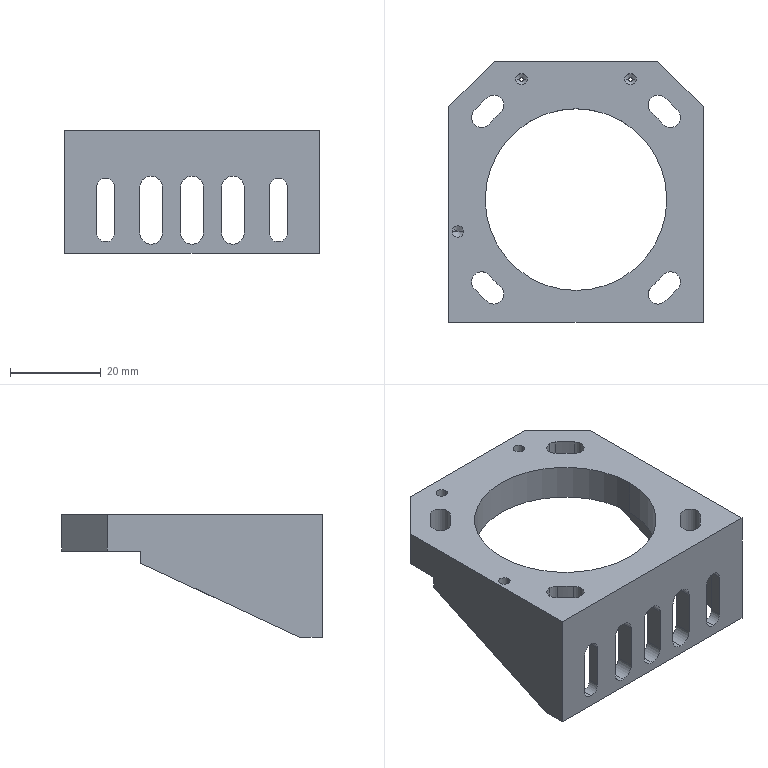Part | 1 solid | 81 faces | box 56 x 57.4 x 27 mm | volume 18700 mm3 | cylinder 47 | plane 28 | cone 6 | commonest cylinder face diameters 4.4 x12 5 x9 2.5 x6 4 x6 6 x4 50.75 x4